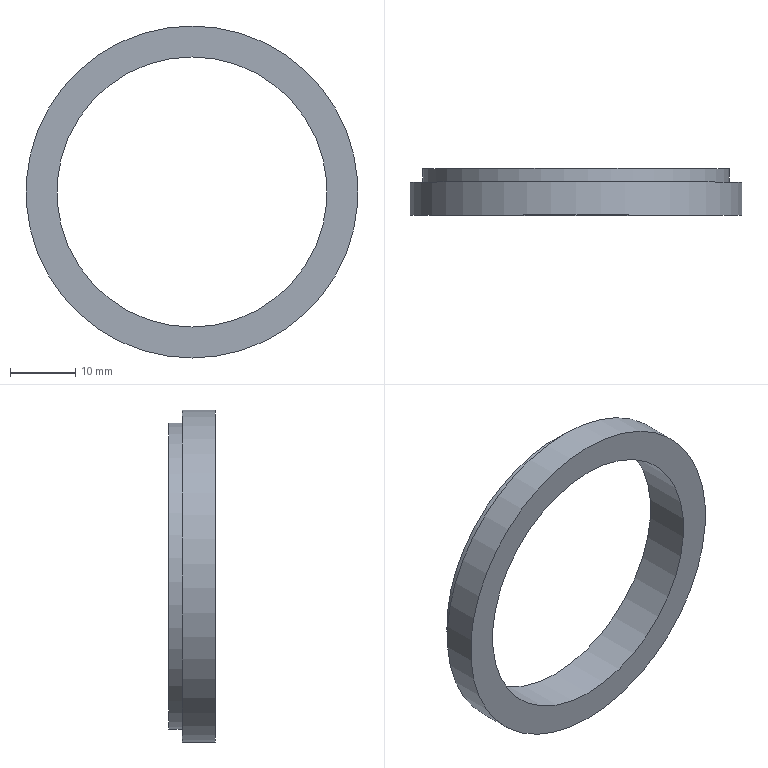Part | NX | features MG0330 trunion parts 24(trunion group) 2 | 1 solid | 6 faces | box 50.927 x 7.144 x 50.927 mm | volume 4298 mm3 | cylinder 3 | plane 3 | commonest cylinder face diameters 41.427 x1 46.99 x1 50.927 x1
STEP:
#1=CARTESIAN_POINT('',(0.,194.786,-25.463));
#2=VERTEX_POINT('',#1);
#3=CARTESIAN_POINT('',(0.,194.786,0.));
#4=DIRECTION('',(0.,-1.,0.));
#5=DIRECTION('',(0.,0.,-1.));
#6=AXIS2_PLACEMENT_3D('',#3,#4,#5);
#7=CIRCLE('',#6,25.463);
#8=EDGE_CURVE('',#2,#2,#7,.T.);
#9=ORIENTED_EDGE('',*,*,#8,.T.);
#10=EDGE_LOOP('',(#9));
#11=FACE_BOUND('',#10,.T.);
#12=CARTESIAN_POINT('',(0.,189.706,-25.463));
#13=VERTEX_POINT('',#12);
#14=CARTESIAN_POINT('',(0.,189.706,0.));
#15=DIRECTION('',(0.,-1.,0.));
#16=DIRECTION('',(0.,0.,-1.));
#17=AXIS2_PLACEMENT_3D('',#14,#15,#16);
#18=CIRCLE('',#17,25.463);
#19=EDGE_CURVE('',#13,#13,#18,.T.);
#20=ORIENTED_EDGE('',*,*,#19,.F.);
#21=EDGE_LOOP('',(#20));
#22=FACE_BOUND('',#21,.T.);
#23=CARTESIAN_POINT('',(0.,0.,0.));
#24=DIRECTION('',(0.,-1.,0.));
#25=DIRECTION('',(0.,0.,-1.));
#26=AXIS2_PLACEMENT_3D('',#23,#24,#25);
#27=CYLINDRICAL_SURFACE('',#26,25.463);
#28=ADVANCED_FACE('',(#11,#22),#27,.T.);
#29=CARTESIAN_POINT('',(0.,194.786,-23.495));
#30=VERTEX_POINT('',#29);
#31=CARTESIAN_POINT('',(0.,194.786,0.));
#32=DIRECTION('',(0.,-1.,0.));
#33=DIRECTION('',(0.,0.,-1.));
#34=AXIS2_PLACEMENT_3D('',#31,#32,#33);
#35=CIRCLE('',#34,23.495);
#36=EDGE_CURVE('',#30,#30,#35,.T.);
#37=ORIENTED_EDGE('',*,*,#36,.T.);
#38=EDGE_LOOP('',(#37));
#39=FACE_BOUND('',#38,.T.);
#40=ORIENTED_EDGE('',*,*,#8,.F.);
#41=EDGE_LOOP('',(#40));
#42=FACE_BOUND('',#41,.T.);
#43=CARTESIAN_POINT('',(25.463,194.786,0.));
#44=DIRECTION('',(0.,1.,0.));
#45=DIRECTION('',(0.,0.,1.));
#46=AXIS2_PLACEMENT_3D('',#43,#44,#45);
#47=PLANE('',#46);
#48=ADVANCED_FACE('',(#39,#42),#47,.T.);
#49=CARTESIAN_POINT('',(0.,196.85,-23.495));
#50=VERTEX_POINT('',#49);
#51=CARTESIAN_POINT('',(0.,196.85,0.));
#52=DIRECTION('',(0.,-1.,0.));
#53=DIRECTION('',(0.,0.,-1.));
#54=AXIS2_PLACEMENT_3D('',#51,#52,#53);
#55=CIRCLE('',#54,23.495);
#56=EDGE_CURVE('',#50,#50,#55,.T.);
#57=ORIENTED_EDGE('',*,*,#56,.T.);
#58=EDGE_LOOP('',(#57));
#59=FACE_BOUND('',#58,.T.);
#60=ORIENTED_EDGE('',*,*,#36,.F.);
#61=EDGE_LOOP('',(#60));
#62=FACE_BOUND('',#61,.T.);
#63=CARTESIAN_POINT('',(0.,0.,0.));
#64=DIRECTION('',(0.,-1.,0.));
#65=DIRECTION('',(0.,0.,-1.));
#66=AXIS2_PLACEMENT_3D('',#63,#64,#65);
#67=CYLINDRICAL_SURFACE('',#66,23.495);
#68=ADVANCED_FACE('',(#59,#62),#67,.T.);
#69=CARTESIAN_POINT('',(0.,196.85,-20.714));
#70=VERTEX_POINT('',#69);
#71=CARTESIAN_POINT('',(0.,196.85,0.));
#72=DIRECTION('',(0.,-1.,0.));
#73=DIRECTION('',(0.,0.,-1.));
#74=AXIS2_PLACEMENT_3D('',#71,#72,#73);
#75=CIRCLE('',#74,20.714);
#76=EDGE_CURVE('',#70,#70,#75,.T.);
#77=ORIENTED_EDGE('',*,*,#76,.T.);
#78=EDGE_LOOP('',(#77));
#79=FACE_BOUND('',#78,.T.);
#80=ORIENTED_EDGE('',*,*,#56,.F.);
#81=EDGE_LOOP('',(#80));
#82=FACE_BOUND('',#81,.T.);
#83=CARTESIAN_POINT('',(20.714,196.85,0.));
#84=DIRECTION('',(0.,1.,0.));
#85=DIRECTION('',(0.,0.,1.));
#86=AXIS2_PLACEMENT_3D('',#83,#84,#85);
#87=PLANE('',#86);
#88=ADVANCED_FACE('',(#79,#82),#87,.T.);
#89=CARTESIAN_POINT('',(0.,189.706,-20.714));
#90=VERTEX_POINT('',#89);
#91=CARTESIAN_POINT('',(0.,189.706,0.));
#92=DIRECTION('',(0.,-1.,0.));
#93=DIRECTION('',(0.,0.,-1.));
#94=AXIS2_PLACEMENT_3D('',#91,#92,#93);
#95=CIRCLE('',#94,20.714);
#96=EDGE_CURVE('',#90,#90,#95,.T.);
#97=ORIENTED_EDGE('',*,*,#96,.T.);
#98=EDGE_LOOP('',(#97));
#99=FACE_BOUND('',#98,.T.);
#100=ORIENTED_EDGE('',*,*,#76,.F.);
#101=EDGE_LOOP('',(#100));
#102=FACE_BOUND('',#101,.T.);
#103=CARTESIAN_POINT('',(0.,0.,0.));
#104=DIRECTION('',(0.,-1.,0.));
#105=DIRECTION('',(0.,0.,-1.));
#106=AXIS2_PLACEMENT_3D('',#103,#104,#105);
#107=CYLINDRICAL_SURFACE('',#106,20.714);
#108=ADVANCED_FACE('',(#99,#102),#107,.F.);
#109=ORIENTED_EDGE('',*,*,#19,.T.);
#110=EDGE_LOOP('',(#109));
#111=FACE_BOUND('',#110,.T.);
#112=ORIENTED_EDGE('',*,*,#96,.F.);
#113=EDGE_LOOP('',(#112));
#114=FACE_BOUND('',#113,.T.);
#115=CARTESIAN_POINT('',(20.714,189.706,0.));
#116=DIRECTION('',(0.,-1.,0.));
#117=DIRECTION('',(0.,0.,-1.));
#118=AXIS2_PLACEMENT_3D('',#115,#116,#117);
#119=PLANE('',#118);
#120=ADVANCED_FACE('',(#111,#114),#119,.T.);
#121=CLOSED_SHELL('',(#28,#48,#68,#88,#108,#120));
#122=MANIFOLD_SOLID_BREP('',#121);
#123=(LENGTH_UNIT()NAMED_UNIT(*)SI_UNIT(.MILLI.,.METRE.));
#124=UNCERTAINTY_MEASURE_WITH_UNIT(LENGTH_MEASURE(0.00001),#123,'','');
#125=(NAMED_UNIT(*)PLANE_ANGLE_UNIT()SI_UNIT($,.RADIAN.));
#126=(NAMED_UNIT(*)SI_UNIT($,.STERADIAN.)SOLID_ANGLE_UNIT());
#127=(GEOMETRIC_REPRESENTATION_CONTEXT(3)GLOBAL_UNCERTAINTY_ASSIGNED_CONTEXT((#124))GLOBAL_UNIT_ASSIGNED_CONTEXT((#123,#125,#126))REPRESENTATION_CONTEXT('',''));
#128=ADVANCED_BREP_SHAPE_REPRESENTATION('',(#122),#127);